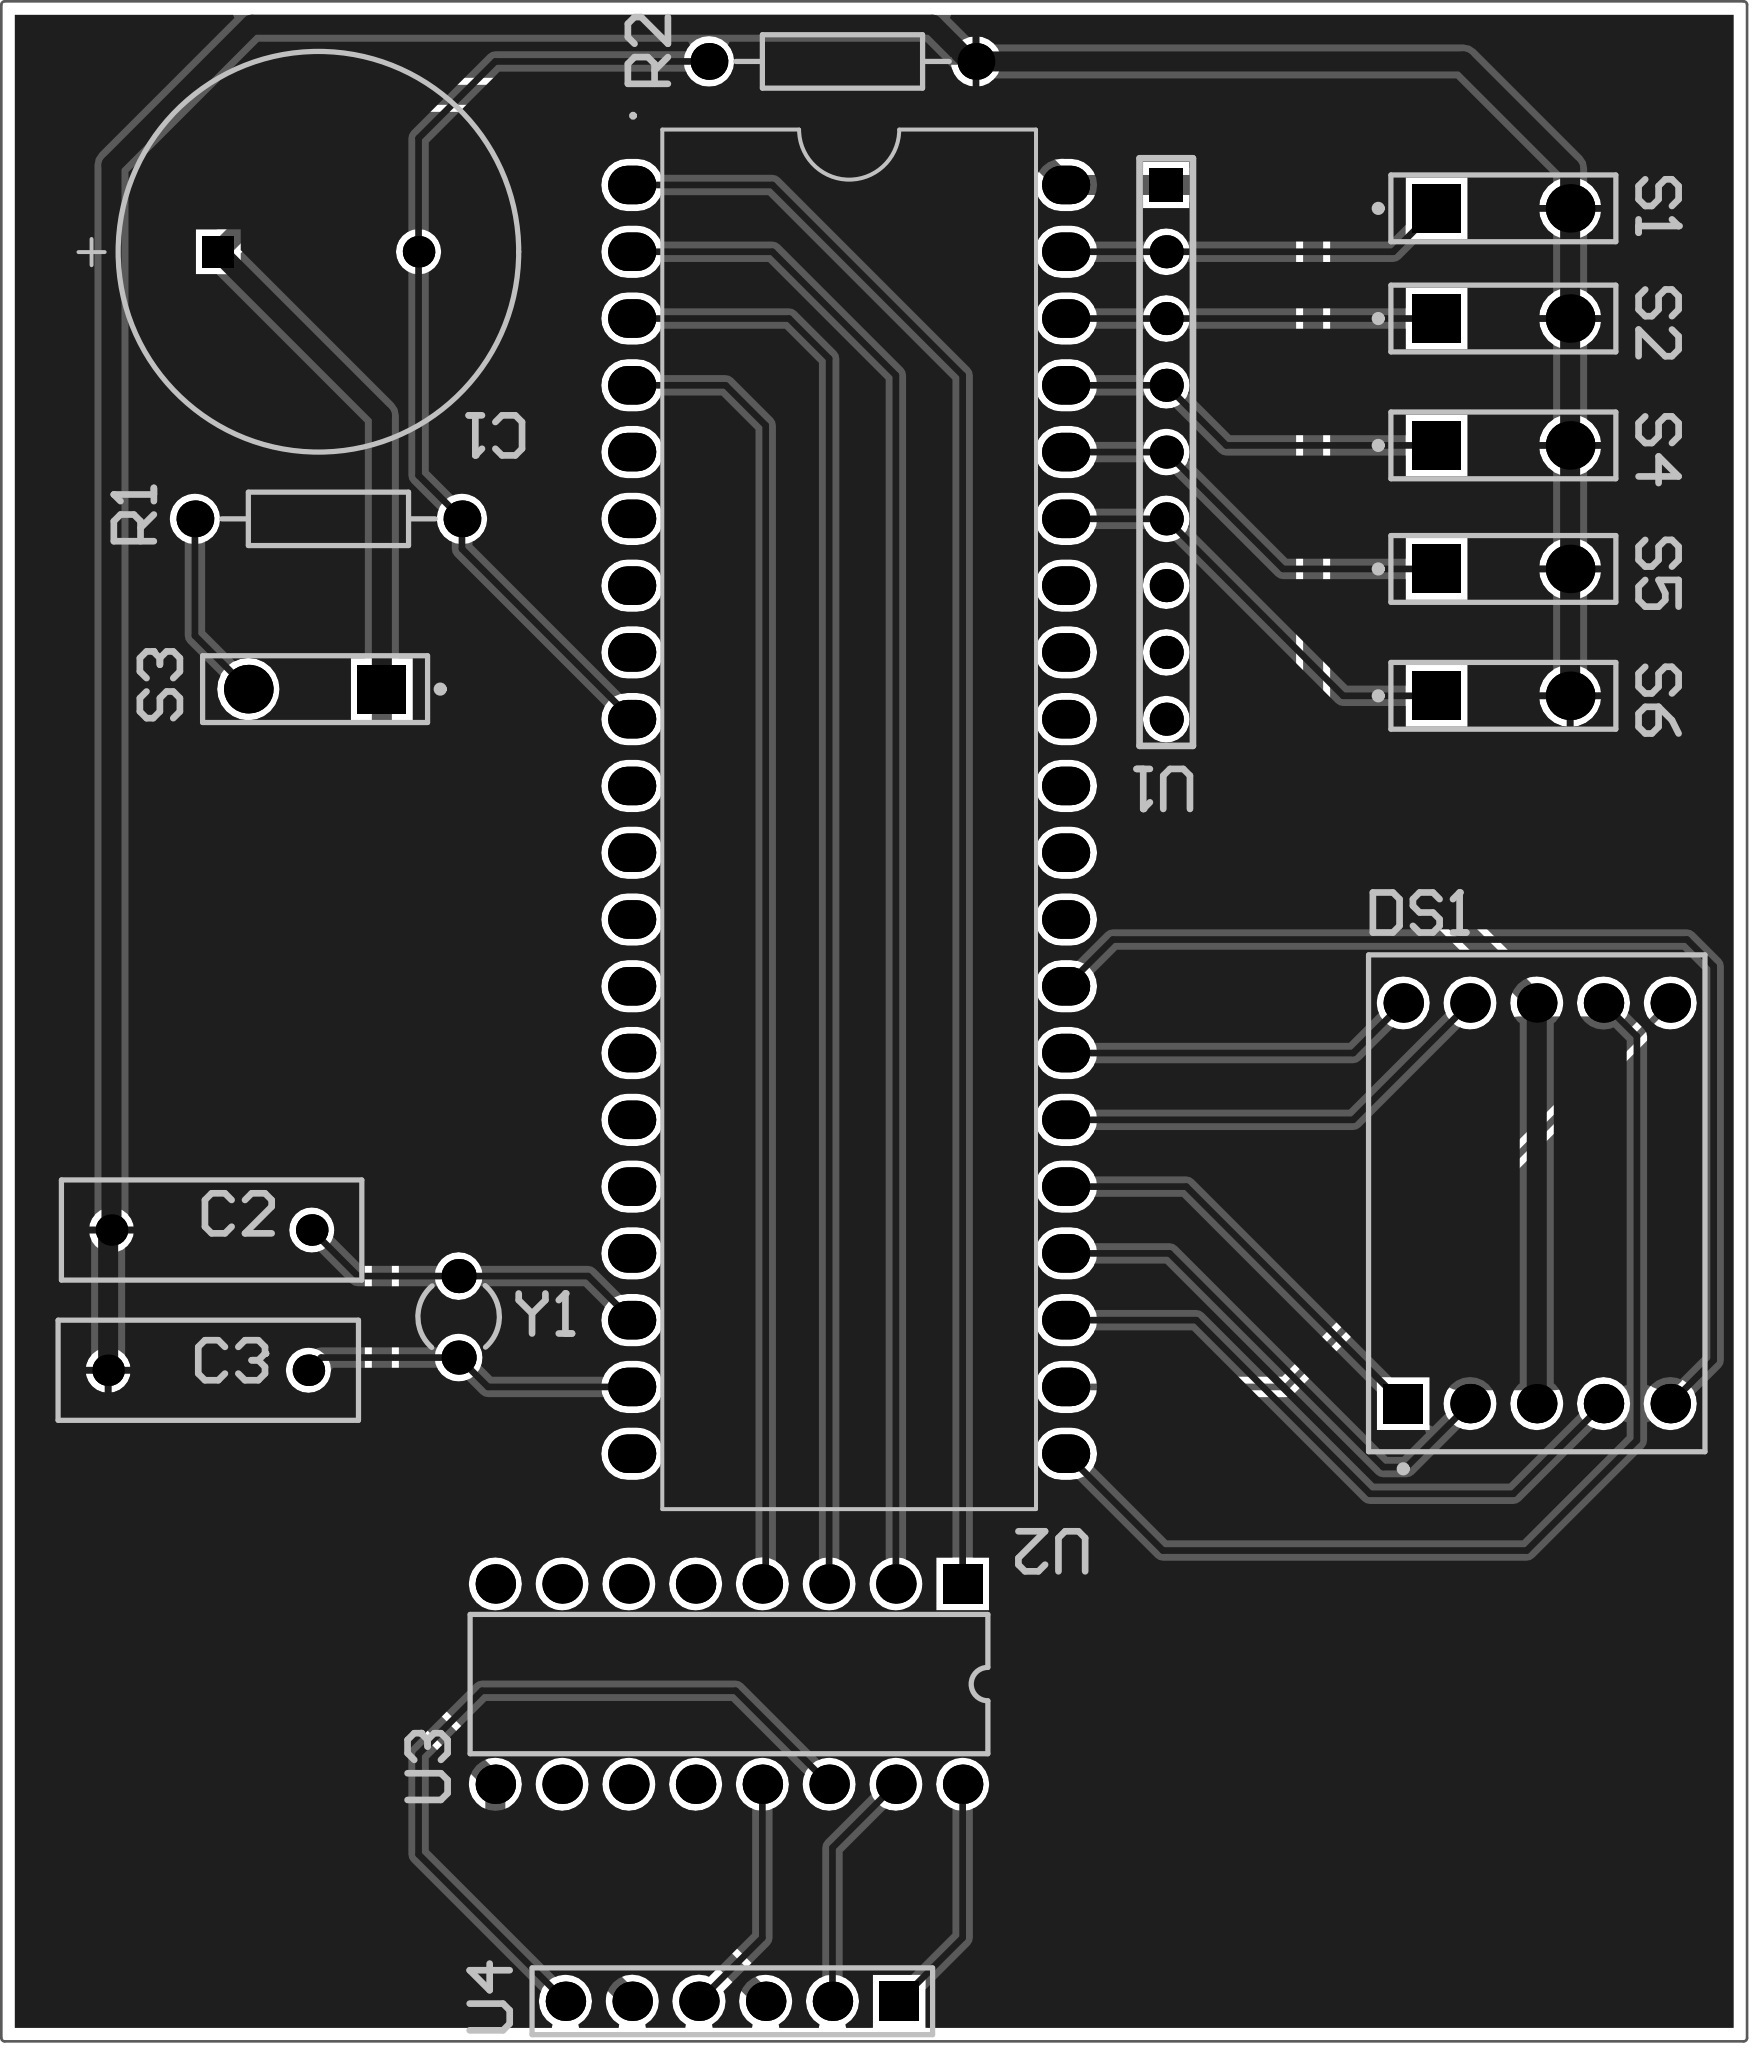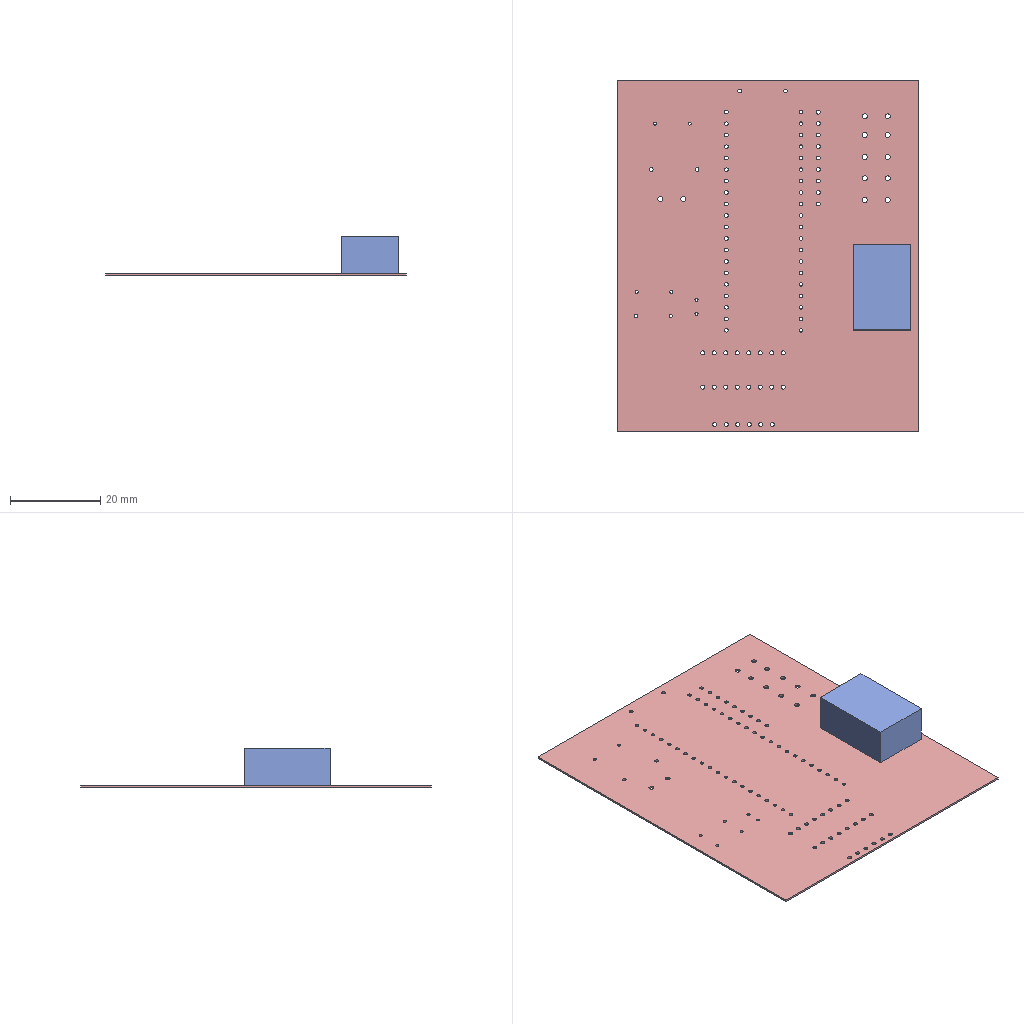Circuit board layout | Altium Designer | box 66.4 x 77.6 x 8.7 mm
Layer stack:
# Altium Designer layer stack of  (unit mm; dielectric type: 0 none, 1 core, 2 prepreg, 3 surface material)
index,name,kind,layer,copper_thickness_mm,dielectric_type,dielectric_thickness_mm,dielectric_material,dielectric_constant
0,Top Paste,other,,,,,,
1,Top Overlay,other,,,,,,
2,Top Solder,dielectric,,,3,0.0102,Solder Resist,3.5
3,Top Layer,copper,Top Layer,0.0356,,,,
4,Dielectric 1,dielectric,,,0,0.32,FR-4,4.8
5,Bottom Layer,copper,Bottom Layer,0.0356,,,,
6,Bottom Solder,dielectric,,,3,0.0102,Solder Resist,3.5
7,Bottom Overlay,other,,,,,,
8,Bottom Paste,other,,,,,,
# drill layer pairs: low layer,high layer
drill_pair,Top Layer,Bottom Layer
Part placement:
Designator,Comment,Layer,Footprint,Center-X(mm),Center-Y(mm),Rotation
Y1,XTAL,TopLayer,R38,83.312,67.437,180
U4,Motor,TopLayer,HDR1X6,93.726,41.402,180
U3,ULN2003A,TopLayer,A16,93.599,53.467,180
U2,STC89C52RC,TopLayer,STC89C52RC,98.171,86.36,270
U1,Resistor network,TopLayer,paizu,110.236,100.33,270
S6,SW-PB,TopLayer,SPST-2,123.063,91.059,360
S5,SW-PB,TopLayer,SPST-2,123.063,95.885,360
S4,SW-PB,TopLayer,SPST-2,123.063,100.584,360
S3,SW-PB,TopLayer,SPST-2,77.851,91.313,180
S2,SW-PB,TopLayer,SPST-2,123.063,105.41,360
S1,SW-PB,TopLayer,SPST-2,123.063,109.601,360
R2,10K,TopLayer,AXIAL-0.4,97.917,115.189,180
R1,220,TopLayer,AXIAL-0.4,78.359,97.79,180
DS1,Dpy Blue-CC,TopLayer,H,124.333,71.755,0
C3,22PF,TopLayer,RAD-0.3,73.787,65.405,360
C2,22PF,TopLayer,RAD-0.3,73.914,70.739,360
C1,10UF,TopLayer,RB7.6-15,77.978,107.95,180
Pad and via stacks:
# Altium Designer via and pad stacks of  (unit mm). Each distinct definition once, with the count of objects using it.
# via: kind,start_layer,end_layer,hole_mm,diameter_mm,mode(0 simple;1 top-mid-bottom;2 full stack),diameter_per_layer,count,example_net
# pad: kind,layer,hole_mm,hole_type(0 round;1 square;2 slot),plating,top_size,top_shape(1 round;2 rect;3 octagon;9 rounded rect),mid_size,bottom_size,mode,footprint,size_per_layer,count,example
pad,Multi-Layer,0.84,0,plated,1.26x1.26,2,1.26x1.26,1.26x1.26,0,paizu,,1,U1.1
pad,Multi-Layer,0.84,0,plated,1.26x1.26,1,1.26x1.26,1.26x1.26,0,paizu,,8,U1.2
pad,Multi-Layer,0.8,0,plated,1.467x1.833,1,1.467x1.833,1.467x1.833,0,STC89C52RC,,40,U2.21
pad,Multi-Layer,1.1,0,plated,1.85x1.85,2,1.85x1.85,1.85x1.85,0,SPST-2,,6,S1.1
pad,Multi-Layer,1.1,0,plated,1.85x1.85,1,1.85x1.85,1.85x1.85,0,SPST-2,,6,S1.2
pad,Multi-Layer,0.85,0,plated,1.4x1.4,1,1.4x1.4,1.4x1.4,0,AXIAL-0.4,,4,R1.1
pad,Multi-Layer,0.7,0,plated,1.2x1.2,2,1.2x1.2,1.2x1.2,0,RB7.6-15,,1,C1.1
pad,Multi-Layer,0.7,0,plated,1.2x1.2,1,1.2x1.2,1.2x1.2,0,RB7.6-15,,1,C1.2
pad,Multi-Layer,0.9,0,plated,1.5x1.5,2,1.5x1.5,1.5x1.5,0,H,,1,DS1.1
pad,Multi-Layer,0.9,0,plated,1.5x1.5,1,1.5x1.5,1.5x1.5,0,H,,9,DS1.2
pad,Multi-Layer,0.7,0,plated,1.2x1.2,1,1.2x1.2,1.2x1.2,0,RAD-0.3,,4,C2.2
pad,Multi-Layer,0.7,0,plated,1.3x1.3,1,1.3x1.3,1.3x1.3,0,R38,,2,Y1.1
pad,Multi-Layer,0.9,0,plated,1.5x1.5,2,1.5x1.5,1.5x1.5,0,HDR1X6,,1,U4.1
pad,Multi-Layer,0.9,0,plated,1.5x1.5,1,1.5x1.5,1.5x1.5,0,HDR1X6,,5,U4.2
pad,Multi-Layer,0.9,0,plated,1.5x1.5,2,1.5x1.5,1.5x1.5,0,A16,,1,U3.1
pad,Multi-Layer,0.9,0,plated,1.5x1.5,1,1.5x1.5,1.5x1.5,0,A16,,15,U3.2
Copper pours:
name,layer,net,type(0 solid;1 hatched;2 none)
Top Layer-No Net,Bottom Layer,GND,0
Top Layer-No Net,Top Layer,GND,0
Design rules, without the lines most boards share:
# Altium Designer design rules of  (exported by Altium Designer, unit mm)
# columns: name | kind | enabled | priority | scope1 | scope2 | descriptor | typed fields (field=value)
SilkToSilkClearance | 55 | enabled | 1 | All | All | Silk to Silk (Clearance=0mil) (All),(All) |
SilkToSolderMaskClearance | 54 | enabled | 1 | IsPad | All | Silk To Solder Mask (Clearance=0mil) (IsPad),(All) |
MinimumSolderMaskSliver | 53 | enabled | 1 | All | All | Minimum Solder Mask Sliver (Gap=0mil) (All),(All) |
HoleToHoleClearance | 52 | enabled | 1 | All | All | Hole To Hole Clearance (Gap=10mil) (All),(All) | gap=0.254
DiffPairsRouting | 51 | enabled | 1 | All | All | Differential Pairs Uncoupled Length using the Gap Constraints (Min=10mil) (Max=10mil) (Prefered=10mil)  and Width Constraints (Min=15mil) (Max=15mil) (Prefered=15mil) (All) |
SolderMaskExpansion | 13 | enabled | 1 | All | All | Solder Mask Expansion (Expansion =4mil) (All) | expansion=0.1016
PasteMaskExpansion | 14 | enabled | 1 | All | All | Paste Mask Expansion (Expansion =0mil) (All) | expansion=0
RoutingVias | 11 | enabled | 1 | All | All | Routing Via (MinHoleWidth=28mil) (MaxHoleWidth=28mil) (PreferredHoleWidth=28mil) (MinWidth=50mil) (MaxWidth=50mil) (PreferedWidth=50mil) (All) | via_min_hole=0.7112 via_max_hole=0.7112 via_preferred_diameter=1.27 via_preferred_hole=0.7112
Width | 2 | enabled | 1 | All | All | Width Constraint (Min=10mil) (Max=30mil) (Preferred=10mil) (All) |
PolygonConnect | 20 | enabled | 1 | All | All | Polygon Connect Rule(Relief Connect )(Conductor Width=10mil) (Relief Angle=90 Angle) (Entries=4) (Air Gap Width=10mil) (All),(All) | connect_style(0=relief,1=direct,2=none)=0 relief_conductor_width=0.254 relief_entries=4
PlaneConnect | 6 | enabled | 1 | All | All | Power Plane Connect Rule(Relief Connect )(Expansion=20mil) (Conductor Width=10mil) (Air Gap=10mil) (Entries=4) (All) | relief_conductor_width=0.254 relief_entries=4 relief_expansion=0.508
Clearance | 0 | enabled | 1 | All | All | Clearance Constraint (Gap=10mil) (All),(All) | gap=0.254
Classes set for this board:
# Altium Designer classes of  (member kind: 0 net, 1 component, 2 from-to, 3 pad, 4 layer, 5 differential pair, 6 design channel, 7 polygon, 8 structure, 9 xSignal)
# columns: class name | member kind | superclass | members
Sheet1 | 1 | no | C1; C2; C3; DS1; R1; R2; S1; S2; S3; S4; S5; S6; U1; U2; U3; U4; Y1;